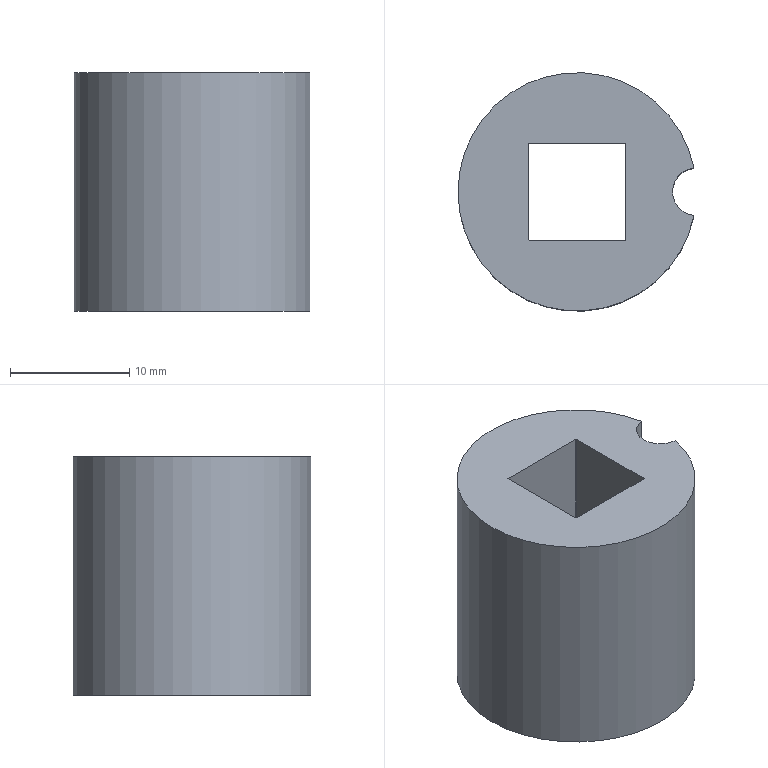Part | NX | features solid 2 | 1 solid | 14 faces | box 19.8 x 20 x 20 mm | volume 4142 mm3 | cylinder 7 | plane 7 | commonest cylinder face diameters 0.04 x4 4 x1 12.6 x1 20 x1
STEP:
#1=CARTESIAN_POINT('',(194.953,202.74,-0.8702));
#2=VERTEX_POINT('',#1);
#3=CARTESIAN_POINT('',(194.953,202.74,19.13));
#4=VERTEX_POINT('',#3);
#5=CARTESIAN_POINT('',(194.953,202.74,9.13));
#6=DIRECTION('',(0.,0.,1.));
#7=VECTOR('',#6,1000.);
#8=LINE('',#5,#7);
#9=EDGE_CURVE('',#2,#4,#8,.T.);
#10=ORIENTED_EDGE('',*,*,#9,.F.);
#11=CARTESIAN_POINT('',(194.953,198.76,-0.8702));
#12=VERTEX_POINT('',#11);
#13=CARTESIAN_POINT('',(185.153,200.75,-0.8702));
#14=DIRECTION('',(0.,0.,1.));
#15=DIRECTION('',(1.,0.,0.));
#16=AXIS2_PLACEMENT_3D('',#13,#14,#15);
#17=CIRCLE('',#16,10.);
#18=EDGE_CURVE('',#2,#12,#17,.T.);
#19=ORIENTED_EDGE('',*,*,#18,.T.);
#20=CARTESIAN_POINT('',(194.953,198.76,19.13));
#21=VERTEX_POINT('',#20);
#22=CARTESIAN_POINT('',(194.953,198.76,9.13));
#23=DIRECTION('',(0.,0.,1.));
#24=VECTOR('',#23,1000.);
#25=LINE('',#22,#24);
#26=EDGE_CURVE('',#21,#12,#25,.F.);
#27=ORIENTED_EDGE('',*,*,#26,.F.);
#28=CARTESIAN_POINT('',(185.153,200.75,19.13));
#29=DIRECTION('',(0.,0.,1.));
#30=DIRECTION('',(1.,0.,0.));
#31=AXIS2_PLACEMENT_3D('',#28,#29,#30);
#32=CIRCLE('',#31,10.);
#33=EDGE_CURVE('',#4,#21,#32,.T.);
#34=ORIENTED_EDGE('',*,*,#33,.F.);
#35=EDGE_LOOP('',(#10,#19,#27,#34));
#36=FACE_BOUND('',#35,.T.);
#37=CARTESIAN_POINT('',(185.153,200.75,-0.8702));
#38=DIRECTION('',(0.,0.,1.));
#39=DIRECTION('',(1.,0.,0.));
#40=AXIS2_PLACEMENT_3D('',#37,#38,#39);
#41=CYLINDRICAL_SURFACE('',#40,10.);
#42=ADVANCED_FACE('',(#36),#41,.T.);
#43=CARTESIAN_POINT('',(191.453,200.75,-0.8702));
#44=VERTEX_POINT('',#43);
#45=CARTESIAN_POINT('',(185.153,200.75,-0.8702));
#46=DIRECTION('',(0.,0.,1.));
#47=DIRECTION('',(1.,0.,0.));
#48=AXIS2_PLACEMENT_3D('',#45,#46,#47);
#49=CIRCLE('',#48,6.3);
#50=EDGE_CURVE('',#44,#44,#49,.T.);
#51=ORIENTED_EDGE('',*,*,#50,.T.);
#52=EDGE_LOOP('',(#51));
#53=FACE_BOUND('',#52,.T.);
#54=ORIENTED_EDGE('',*,*,#18,.F.);
#55=CARTESIAN_POINT('',(195.153,200.75,-0.8702));
#56=DIRECTION('',(0.,0.,1.));
#57=DIRECTION('',(1.,0.,0.));
#58=AXIS2_PLACEMENT_3D('',#55,#56,#57);
#59=CIRCLE('',#58,2.);
#60=EDGE_CURVE('',#2,#12,#59,.T.);
#61=ORIENTED_EDGE('',*,*,#60,.T.);
#62=EDGE_LOOP('',(#54,#61));
#63=FACE_BOUND('',#62,.T.);
#64=CARTESIAN_POINT('',(185.153,200.75,-0.8702));
#65=DIRECTION('',(0.,0.,1.));
#66=DIRECTION('',(1.,0.,0.));
#67=AXIS2_PLACEMENT_3D('',#64,#65,#66);
#68=PLANE('',#67);
#69=ADVANCED_FACE('',(#53,#63),#68,.F.);
#70=CARTESIAN_POINT('',(181.103,204.78,19.13));
#71=VERTEX_POINT('',#70);
#72=CARTESIAN_POINT('',(181.103,196.72,19.13));
#73=VERTEX_POINT('',#72);
#74=CARTESIAN_POINT('',(181.103,204.8,19.13));
#75=DIRECTION('',(0.,-1.,0.));
#76=VECTOR('',#75,1000.);
#77=LINE('',#74,#76);
#78=EDGE_CURVE('',#71,#73,#77,.T.);
#79=ORIENTED_EDGE('',*,*,#78,.F.);
#80=CARTESIAN_POINT('',(181.123,204.8,19.13));
#81=VERTEX_POINT('',#80);
#82=CARTESIAN_POINT('',(181.123,204.78,19.13));
#83=DIRECTION('',(0.,0.,1.));
#84=DIRECTION('',(1.,0.,0.));
#85=AXIS2_PLACEMENT_3D('',#82,#83,#84);
#86=CIRCLE('',#85,0.02);
#87=EDGE_CURVE('',#71,#81,#86,.F.);
#88=ORIENTED_EDGE('',*,*,#87,.T.);
#89=CARTESIAN_POINT('',(189.183,204.8,19.13));
#90=VERTEX_POINT('',#89);
#91=CARTESIAN_POINT('',(189.203,204.8,19.13));
#92=DIRECTION('',(-1.,0.,0.));
#93=VECTOR('',#92,1000.);
#94=LINE('',#91,#93);
#95=EDGE_CURVE('',#90,#81,#94,.T.);
#96=ORIENTED_EDGE('',*,*,#95,.F.);
#97=CARTESIAN_POINT('',(189.203,204.78,19.13));
#98=VERTEX_POINT('',#97);
#99=CARTESIAN_POINT('',(189.183,204.78,19.13));
#100=DIRECTION('',(0.,0.,1.));
#101=DIRECTION('',(1.,0.,0.));
#102=AXIS2_PLACEMENT_3D('',#99,#100,#101);
#103=CIRCLE('',#102,0.02);
#104=EDGE_CURVE('',#90,#98,#103,.F.);
#105=ORIENTED_EDGE('',*,*,#104,.T.);
#106=CARTESIAN_POINT('',(189.203,196.72,19.13));
#107=VERTEX_POINT('',#106);
#108=CARTESIAN_POINT('',(189.203,204.8,19.13));
#109=DIRECTION('',(0.,-1.,0.));
#110=VECTOR('',#109,1000.);
#111=LINE('',#108,#110);
#112=EDGE_CURVE('',#98,#107,#111,.T.);
#113=ORIENTED_EDGE('',*,*,#112,.T.);
#114=CARTESIAN_POINT('',(189.183,196.7,19.13));
#115=VERTEX_POINT('',#114);
#116=CARTESIAN_POINT('',(189.183,196.72,19.13));
#117=DIRECTION('',(0.,0.,1.));
#118=DIRECTION('',(1.,0.,0.));
#119=AXIS2_PLACEMENT_3D('',#116,#117,#118);
#120=CIRCLE('',#119,0.02);
#121=EDGE_CURVE('',#107,#115,#120,.F.);
#122=ORIENTED_EDGE('',*,*,#121,.T.);
#123=CARTESIAN_POINT('',(181.123,196.7,19.13));
#124=VERTEX_POINT('',#123);
#125=CARTESIAN_POINT('',(181.103,196.7,19.13));
#126=DIRECTION('',(1.,0.,0.));
#127=VECTOR('',#126,1000.);
#128=LINE('',#125,#127);
#129=EDGE_CURVE('',#124,#115,#128,.T.);
#130=ORIENTED_EDGE('',*,*,#129,.F.);
#131=CARTESIAN_POINT('',(181.123,196.72,19.13));
#132=DIRECTION('',(0.,0.,1.));
#133=DIRECTION('',(1.,0.,0.));
#134=AXIS2_PLACEMENT_3D('',#131,#132,#133);
#135=CIRCLE('',#134,0.02);
#136=EDGE_CURVE('',#124,#73,#135,.F.);
#137=ORIENTED_EDGE('',*,*,#136,.T.);
#138=EDGE_LOOP('',(#79,#88,#96,#105,#113,#122,#130,#137));
#139=FACE_BOUND('',#138,.T.);
#140=CARTESIAN_POINT('',(195.153,200.75,19.13));
#141=DIRECTION('',(0.,0.,1.));
#142=DIRECTION('',(1.,0.,0.));
#143=AXIS2_PLACEMENT_3D('',#140,#141,#142);
#144=CIRCLE('',#143,2.);
#145=EDGE_CURVE('',#4,#21,#144,.T.);
#146=ORIENTED_EDGE('',*,*,#145,.F.);
#147=ORIENTED_EDGE('',*,*,#33,.T.);
#148=EDGE_LOOP('',(#146,#147));
#149=FACE_BOUND('',#148,.T.);
#150=CARTESIAN_POINT('',(185.153,200.75,19.13));
#151=DIRECTION('',(0.,0.,1.));
#152=DIRECTION('',(1.,0.,0.));
#153=AXIS2_PLACEMENT_3D('',#150,#151,#152);
#154=PLANE('',#153);
#155=ADVANCED_FACE('',(#139,#149),#154,.T.);
#156=ORIENTED_EDGE('',*,*,#50,.F.);
#157=EDGE_LOOP('',(#156));
#158=FACE_BOUND('',#157,.T.);
#159=CARTESIAN_POINT('',(191.453,200.75,11.13));
#160=VERTEX_POINT('',#159);
#161=CARTESIAN_POINT('',(185.153,200.75,11.13));
#162=DIRECTION('',(0.,0.,1.));
#163=DIRECTION('',(1.,0.,0.));
#164=AXIS2_PLACEMENT_3D('',#161,#162,#163);
#165=CIRCLE('',#164,6.3);
#166=EDGE_CURVE('',#160,#160,#165,.T.);
#167=ORIENTED_EDGE('',*,*,#166,.T.);
#168=EDGE_LOOP('',(#167));
#169=FACE_BOUND('',#168,.T.);
#170=CARTESIAN_POINT('',(185.153,200.75,-0.8702));
#171=DIRECTION('',(0.,0.,1.));
#172=DIRECTION('',(1.,0.,0.));
#173=AXIS2_PLACEMENT_3D('',#170,#171,#172);
#174=CYLINDRICAL_SURFACE('',#173,6.3);
#175=ADVANCED_FACE('',(#158,#169),#174,.F.);
#176=CARTESIAN_POINT('',(189.203,204.78,11.13));
#177=VERTEX_POINT('',#176);
#178=CARTESIAN_POINT('',(189.203,196.72,11.13));
#179=VERTEX_POINT('',#178);
#180=CARTESIAN_POINT('',(189.203,200.75,11.13));
#181=DIRECTION('',(0.,-1.,0.));
#182=VECTOR('',#181,1000.);
#183=LINE('',#180,#182);
#184=EDGE_CURVE('',#177,#179,#183,.T.);
#185=ORIENTED_EDGE('',*,*,#184,.F.);
#186=CARTESIAN_POINT('',(189.183,204.8,11.13));
#187=VERTEX_POINT('',#186);
#188=CARTESIAN_POINT('',(189.183,204.78,11.13));
#189=DIRECTION('',(0.,0.,1.));
#190=DIRECTION('',(1.,0.,0.));
#191=AXIS2_PLACEMENT_3D('',#188,#189,#190);
#192=CIRCLE('',#191,0.02);
#193=EDGE_CURVE('',#177,#187,#192,.T.);
#194=ORIENTED_EDGE('',*,*,#193,.T.);
#195=CARTESIAN_POINT('',(181.123,204.8,11.13));
#196=VERTEX_POINT('',#195);
#197=CARTESIAN_POINT('',(185.153,204.8,11.13));
#198=DIRECTION('',(-1.,0.,0.));
#199=VECTOR('',#198,1000.);
#200=LINE('',#197,#199);
#201=EDGE_CURVE('',#187,#196,#200,.T.);
#202=ORIENTED_EDGE('',*,*,#201,.T.);
#203=CARTESIAN_POINT('',(181.103,204.78,11.13));
#204=VERTEX_POINT('',#203);
#205=CARTESIAN_POINT('',(181.123,204.78,11.13));
#206=DIRECTION('',(0.,0.,1.));
#207=DIRECTION('',(1.,0.,0.));
#208=AXIS2_PLACEMENT_3D('',#205,#206,#207);
#209=CIRCLE('',#208,0.02);
#210=EDGE_CURVE('',#196,#204,#209,.T.);
#211=ORIENTED_EDGE('',*,*,#210,.T.);
#212=CARTESIAN_POINT('',(181.103,196.72,11.13));
#213=VERTEX_POINT('',#212);
#214=CARTESIAN_POINT('',(181.103,200.75,11.13));
#215=DIRECTION('',(0.,-1.,0.));
#216=VECTOR('',#215,1000.);
#217=LINE('',#214,#216);
#218=EDGE_CURVE('',#204,#213,#217,.T.);
#219=ORIENTED_EDGE('',*,*,#218,.T.);
#220=CARTESIAN_POINT('',(181.123,196.7,11.13));
#221=VERTEX_POINT('',#220);
#222=CARTESIAN_POINT('',(181.123,196.72,11.13));
#223=DIRECTION('',(0.,0.,1.));
#224=DIRECTION('',(1.,0.,0.));
#225=AXIS2_PLACEMENT_3D('',#222,#223,#224);
#226=CIRCLE('',#225,0.02);
#227=EDGE_CURVE('',#213,#221,#226,.T.);
#228=ORIENTED_EDGE('',*,*,#227,.T.);
#229=CARTESIAN_POINT('',(189.183,196.7,11.13));
#230=VERTEX_POINT('',#229);
#231=CARTESIAN_POINT('',(185.153,196.7,11.13));
#232=DIRECTION('',(1.,0.,0.));
#233=VECTOR('',#232,1000.);
#234=LINE('',#231,#233);
#235=EDGE_CURVE('',#221,#230,#234,.T.);
#236=ORIENTED_EDGE('',*,*,#235,.T.);
#237=CARTESIAN_POINT('',(189.183,196.72,11.13));
#238=DIRECTION('',(0.,0.,1.));
#239=DIRECTION('',(1.,0.,0.));
#240=AXIS2_PLACEMENT_3D('',#237,#238,#239);
#241=CIRCLE('',#240,0.02);
#242=EDGE_CURVE('',#230,#179,#241,.T.);
#243=ORIENTED_EDGE('',*,*,#242,.T.);
#244=EDGE_LOOP('',(#185,#194,#202,#211,#219,#228,#236,#243));
#245=FACE_BOUND('',#244,.T.);
#246=ORIENTED_EDGE('',*,*,#166,.F.);
#247=EDGE_LOOP('',(#246));
#248=FACE_BOUND('',#247,.T.);
#249=CARTESIAN_POINT('',(185.153,200.75,11.13));
#250=DIRECTION('',(0.,0.,1.));
#251=DIRECTION('',(1.,0.,0.));
#252=AXIS2_PLACEMENT_3D('',#249,#250,#251);
#253=PLANE('',#252);
#254=ADVANCED_FACE('',(#245,#248),#253,.F.);
#255=ORIENTED_EDGE('',*,*,#9,.T.);
#256=ORIENTED_EDGE('',*,*,#145,.T.);
#257=ORIENTED_EDGE('',*,*,#26,.T.);
#258=ORIENTED_EDGE('',*,*,#60,.F.);
#259=EDGE_LOOP('',(#255,#256,#257,#258));
#260=FACE_BOUND('',#259,.T.);
#261=CARTESIAN_POINT('',(195.153,200.75,-0.8702));
#262=DIRECTION('',(0.,0.,1.));
#263=DIRECTION('',(1.,0.,0.));
#264=AXIS2_PLACEMENT_3D('',#261,#262,#263);
#265=CYLINDRICAL_SURFACE('',#264,2.);
#266=ADVANCED_FACE('',(#260),#265,.F.);
#267=ORIENTED_EDGE('',*,*,#78,.T.);
#268=CARTESIAN_POINT('',(181.103,196.72,11.13));
#269=DIRECTION('',(0.,0.,1.));
#270=VECTOR('',#269,1000.);
#271=LINE('',#268,#270);
#272=EDGE_CURVE('',#73,#213,#271,.F.);
#273=ORIENTED_EDGE('',*,*,#272,.T.);
#274=ORIENTED_EDGE('',*,*,#218,.F.);
#275=CARTESIAN_POINT('',(181.103,204.78,19.13));
#276=DIRECTION('',(0.,0.,1.));
#277=VECTOR('',#276,1000.);
#278=LINE('',#275,#277);
#279=EDGE_CURVE('',#204,#71,#278,.T.);
#280=ORIENTED_EDGE('',*,*,#279,.T.);
#281=EDGE_LOOP('',(#267,#273,#274,#280));
#282=FACE_BOUND('',#281,.T.);
#283=CARTESIAN_POINT('',(181.103,204.8,-0.8702));
#284=DIRECTION('',(-1.,0.,0.));
#285=DIRECTION('',(0.,0.,1.));
#286=AXIS2_PLACEMENT_3D('',#283,#284,#285);
#287=PLANE('',#286);
#288=ADVANCED_FACE('',(#282),#287,.F.);
#289=ORIENTED_EDGE('',*,*,#129,.T.);
#290=CARTESIAN_POINT('',(189.183,196.7,-0.8702));
#291=DIRECTION('',(0.,0.,1.));
#292=VECTOR('',#291,1000.);
#293=LINE('',#290,#292);
#294=EDGE_CURVE('',#115,#230,#293,.F.);
#295=ORIENTED_EDGE('',*,*,#294,.T.);
#296=ORIENTED_EDGE('',*,*,#235,.F.);
#297=CARTESIAN_POINT('',(181.123,196.7,19.13));
#298=DIRECTION('',(0.,0.,1.));
#299=VECTOR('',#298,1000.);
#300=LINE('',#297,#299);
#301=EDGE_CURVE('',#221,#124,#300,.T.);
#302=ORIENTED_EDGE('',*,*,#301,.T.);
#303=EDGE_LOOP('',(#289,#295,#296,#302));
#304=FACE_BOUND('',#303,.T.);
#305=CARTESIAN_POINT('',(181.103,196.7,-0.8702));
#306=DIRECTION('',(0.,-1.,0.));
#307=DIRECTION('',(0.,0.,-1.));
#308=AXIS2_PLACEMENT_3D('',#305,#306,#307);
#309=PLANE('',#308);
#310=ADVANCED_FACE('',(#304),#309,.F.);
#311=ORIENTED_EDGE('',*,*,#112,.F.);
#312=CARTESIAN_POINT('',(189.203,204.78,-0.8702));
#313=DIRECTION('',(0.,0.,1.));
#314=VECTOR('',#313,1000.);
#315=LINE('',#312,#314);
#316=EDGE_CURVE('',#98,#177,#315,.F.);
#317=ORIENTED_EDGE('',*,*,#316,.T.);
#318=ORIENTED_EDGE('',*,*,#184,.T.);
#319=CARTESIAN_POINT('',(189.203,196.72,-0.8702));
#320=DIRECTION('',(0.,0.,1.));
#321=VECTOR('',#320,1000.);
#322=LINE('',#319,#321);
#323=EDGE_CURVE('',#179,#107,#322,.T.);
#324=ORIENTED_EDGE('',*,*,#323,.T.);
#325=EDGE_LOOP('',(#311,#317,#318,#324));
#326=FACE_BOUND('',#325,.T.);
#327=CARTESIAN_POINT('',(189.203,204.8,-0.8702));
#328=DIRECTION('',(-1.,0.,0.));
#329=DIRECTION('',(0.,0.,1.));
#330=AXIS2_PLACEMENT_3D('',#327,#328,#329);
#331=PLANE('',#330);
#332=ADVANCED_FACE('',(#326),#331,.T.);
#333=ORIENTED_EDGE('',*,*,#201,.F.);
#334=CARTESIAN_POINT('',(189.183,204.8,-0.8702));
#335=DIRECTION('',(0.,0.,1.));
#336=VECTOR('',#335,1000.);
#337=LINE('',#334,#336);
#338=EDGE_CURVE('',#187,#90,#337,.T.);
#339=ORIENTED_EDGE('',*,*,#338,.T.);
#340=ORIENTED_EDGE('',*,*,#95,.T.);
#341=CARTESIAN_POINT('',(181.123,204.8,11.13));
#342=DIRECTION('',(0.,0.,1.));
#343=VECTOR('',#342,1000.);
#344=LINE('',#341,#343);
#345=EDGE_CURVE('',#81,#196,#344,.F.);
#346=ORIENTED_EDGE('',*,*,#345,.T.);
#347=EDGE_LOOP('',(#333,#339,#340,#346));
#348=FACE_BOUND('',#347,.T.);
#349=CARTESIAN_POINT('',(189.203,204.8,-0.8702));
#350=DIRECTION('',(0.,1.,0.));
#351=DIRECTION('',(0.,0.,1.));
#352=AXIS2_PLACEMENT_3D('',#349,#350,#351);
#353=PLANE('',#352);
#354=ADVANCED_FACE('',(#348),#353,.F.);
#355=ORIENTED_EDGE('',*,*,#193,.F.);
#356=ORIENTED_EDGE('',*,*,#316,.F.);
#357=ORIENTED_EDGE('',*,*,#104,.F.);
#358=ORIENTED_EDGE('',*,*,#338,.F.);
#359=EDGE_LOOP('',(#355,#356,#357,#358));
#360=FACE_BOUND('',#359,.T.);
#361=CARTESIAN_POINT('',(189.183,204.78,-0.8702));
#362=DIRECTION('',(0.,0.,1.));
#363=DIRECTION('',(1.,0.,0.));
#364=AXIS2_PLACEMENT_3D('',#361,#362,#363);
#365=CYLINDRICAL_SURFACE('',#364,0.02);
#366=ADVANCED_FACE('',(#360),#365,.F.);
#367=ORIENTED_EDGE('',*,*,#242,.F.);
#368=ORIENTED_EDGE('',*,*,#294,.F.);
#369=ORIENTED_EDGE('',*,*,#121,.F.);
#370=ORIENTED_EDGE('',*,*,#323,.F.);
#371=EDGE_LOOP('',(#367,#368,#369,#370));
#372=FACE_BOUND('',#371,.T.);
#373=CARTESIAN_POINT('',(189.183,196.72,-0.8702));
#374=DIRECTION('',(0.,0.,1.));
#375=DIRECTION('',(1.,0.,0.));
#376=AXIS2_PLACEMENT_3D('',#373,#374,#375);
#377=CYLINDRICAL_SURFACE('',#376,0.02);
#378=ADVANCED_FACE('',(#372),#377,.F.);
#379=ORIENTED_EDGE('',*,*,#227,.F.);
#380=ORIENTED_EDGE('',*,*,#272,.F.);
#381=ORIENTED_EDGE('',*,*,#136,.F.);
#382=ORIENTED_EDGE('',*,*,#301,.F.);
#383=EDGE_LOOP('',(#379,#380,#381,#382));
#384=FACE_BOUND('',#383,.T.);
#385=CARTESIAN_POINT('',(181.123,196.72,-0.8702));
#386=DIRECTION('',(0.,0.,-1.));
#387=DIRECTION('',(-1.,0.,0.));
#388=AXIS2_PLACEMENT_3D('',#385,#386,#387);
#389=CYLINDRICAL_SURFACE('',#388,0.02);
#390=ADVANCED_FACE('',(#384),#389,.F.);
#391=ORIENTED_EDGE('',*,*,#210,.F.);
#392=ORIENTED_EDGE('',*,*,#345,.F.);
#393=ORIENTED_EDGE('',*,*,#87,.F.);
#394=ORIENTED_EDGE('',*,*,#279,.F.);
#395=EDGE_LOOP('',(#391,#392,#393,#394));
#396=FACE_BOUND('',#395,.T.);
#397=CARTESIAN_POINT('',(181.123,204.78,-0.8702));
#398=DIRECTION('',(0.,0.,-1.));
#399=DIRECTION('',(-1.,0.,0.));
#400=AXIS2_PLACEMENT_3D('',#397,#398,#399);
#401=CYLINDRICAL_SURFACE('',#400,0.02);
#402=ADVANCED_FACE('',(#396),#401,.F.);
#403=CLOSED_SHELL('',(#42,#69,#155,#175,#254,#266,#288,#310,#332,#354,#366,#378,#390,#402));
#404=MANIFOLD_SOLID_BREP('',#403);
#405=(LENGTH_UNIT()NAMED_UNIT(*)SI_UNIT(.MILLI.,.METRE.));
#406=UNCERTAINTY_MEASURE_WITH_UNIT(LENGTH_MEASURE(0.00001),#405,'','');
#407=(NAMED_UNIT(*)PLANE_ANGLE_UNIT()SI_UNIT($,.RADIAN.));
#408=(NAMED_UNIT(*)SI_UNIT($,.STERADIAN.)SOLID_ANGLE_UNIT());
#409=(GEOMETRIC_REPRESENTATION_CONTEXT(3)GLOBAL_UNCERTAINTY_ASSIGNED_CONTEXT((#406))GLOBAL_UNIT_ASSIGNED_CONTEXT((#405,#407,#408))REPRESENTATION_CONTEXT('',''));
#410=ADVANCED_BREP_SHAPE_REPRESENTATION('',(#404),#409);